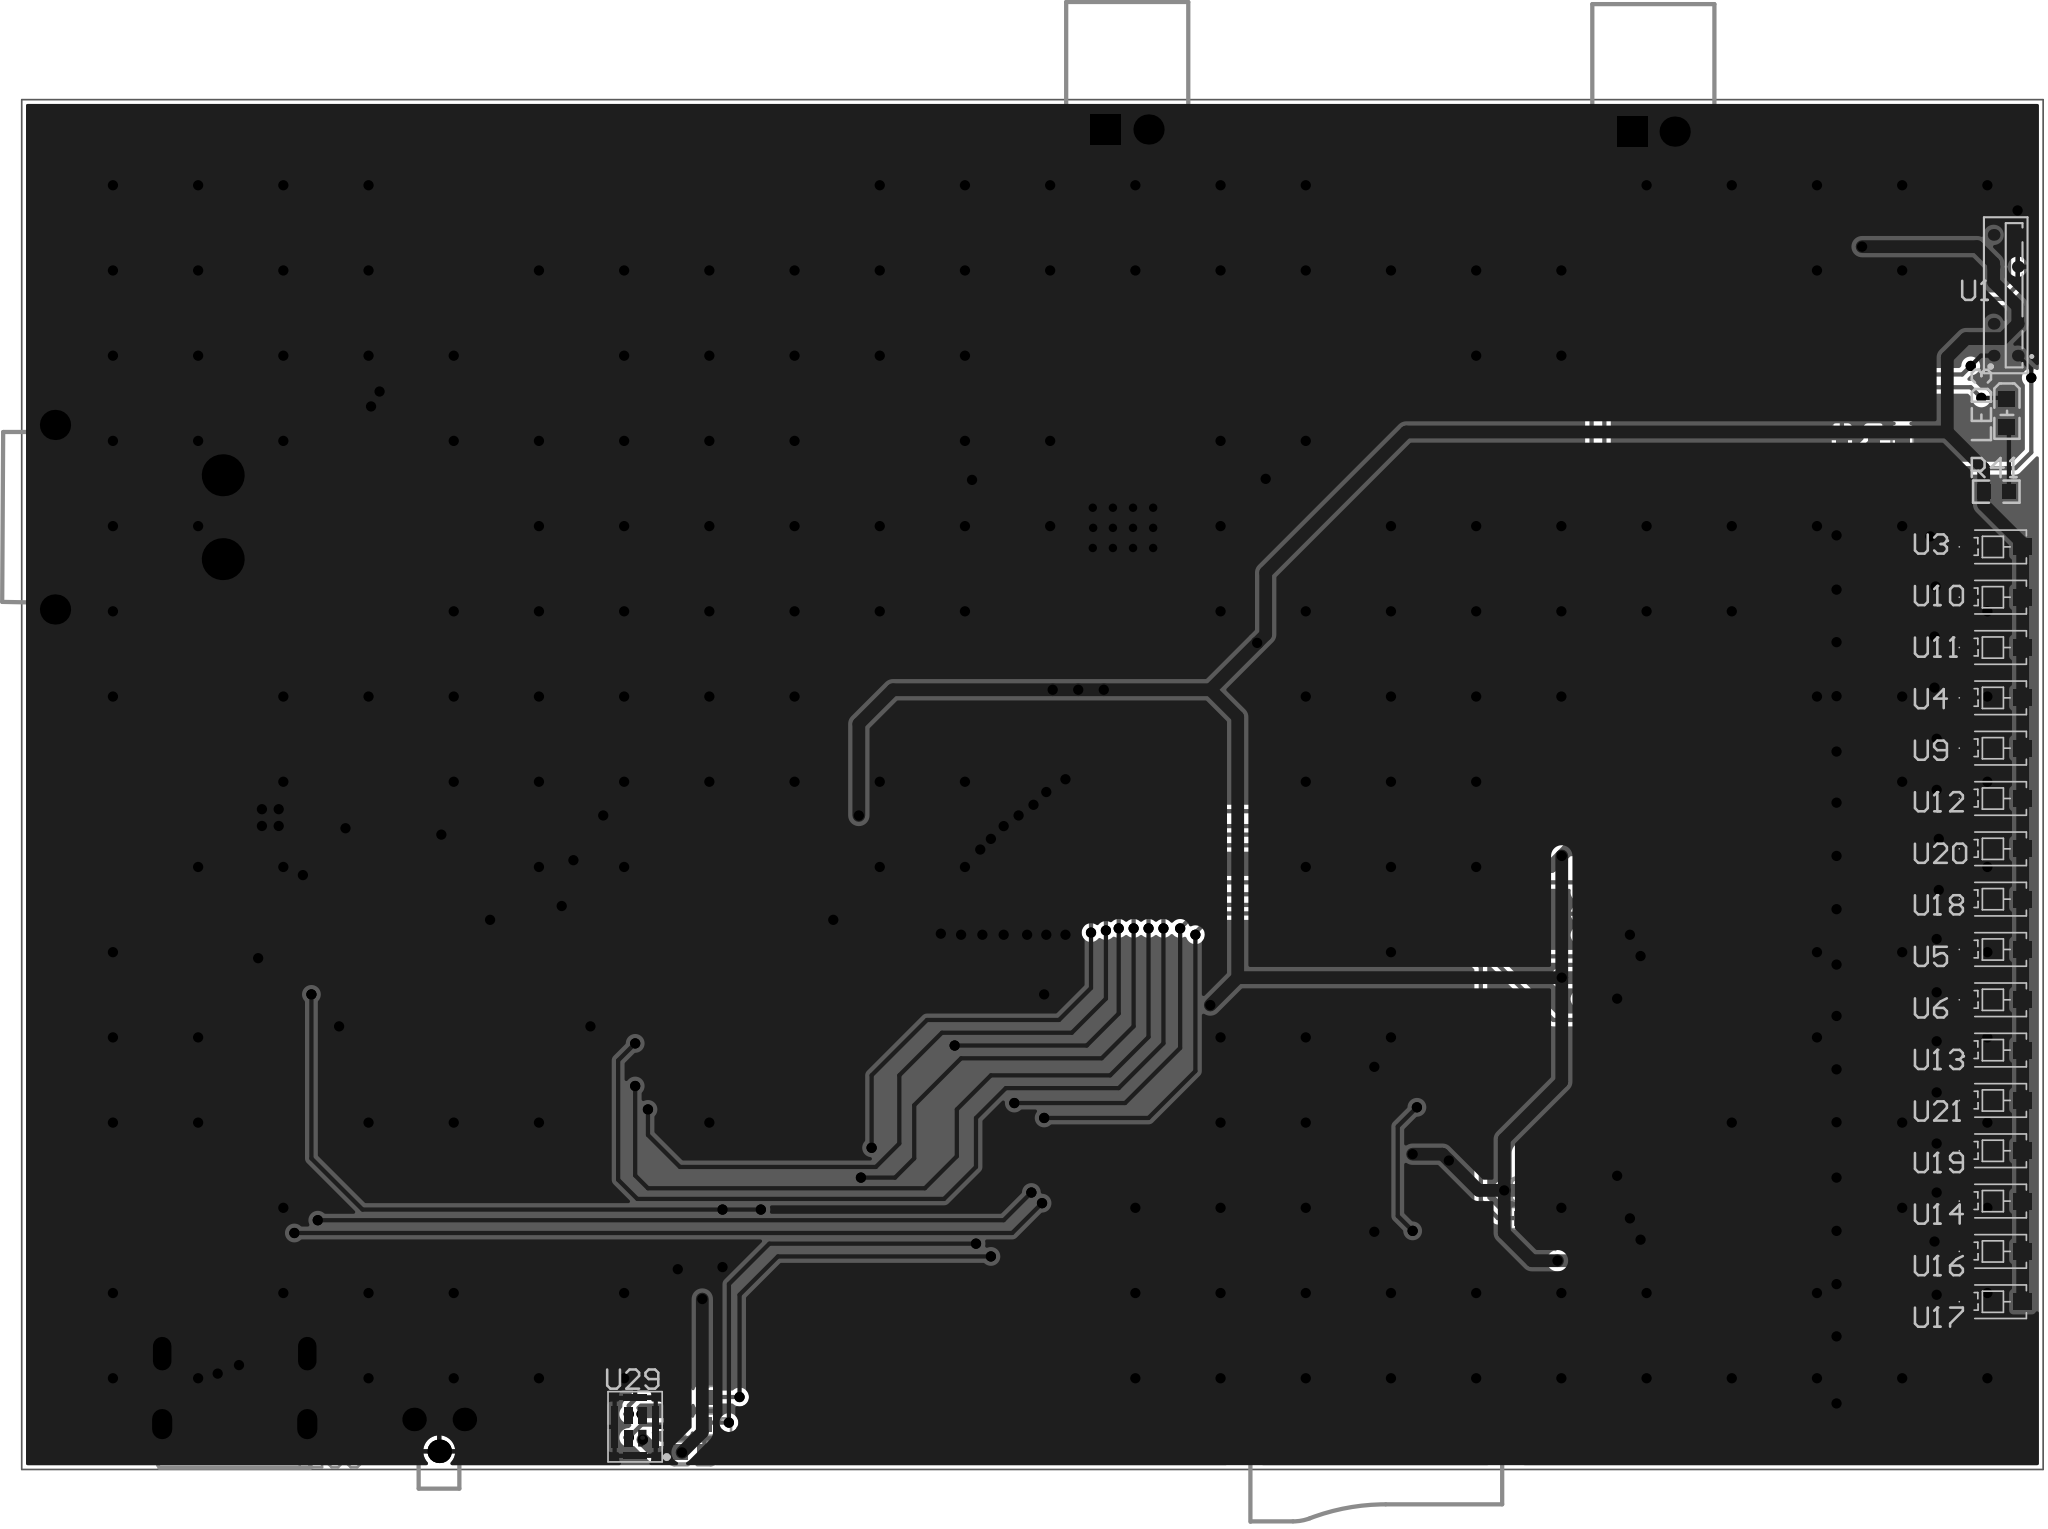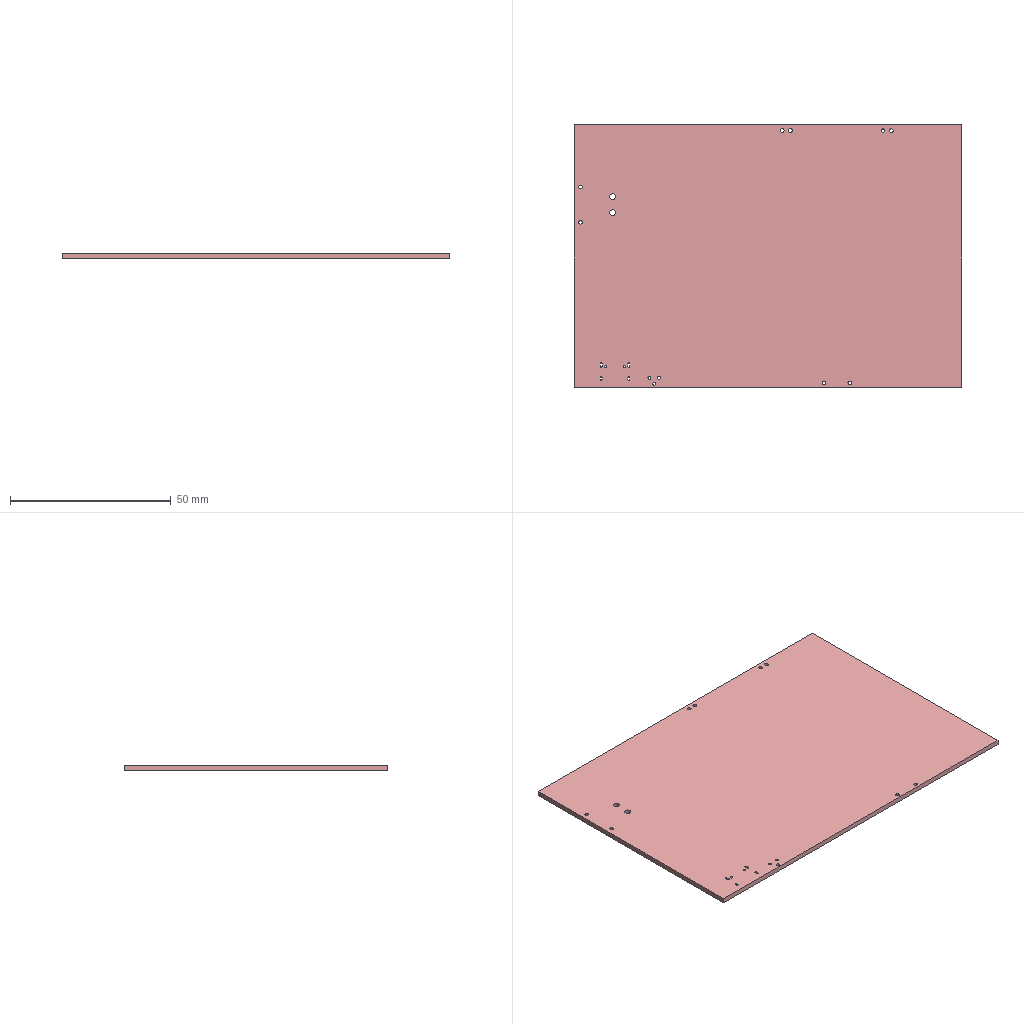Circuit board layout | Altium Designer | box 120.5 x 81.7 x 1.6 mm
Layer stack:
# Altium Designer layer stack of  (unit mm; dielectric type: 0 none, 1 core, 2 prepreg, 3 surface material)
index,name,kind,layer,copper_thickness_mm,dielectric_type,dielectric_thickness_mm,dielectric_material,dielectric_constant
0,Top Paste Mask Layer,other,,,,,,
1,Top Silkscreen Layer,other,,,,,,
2,Top Solder Mask Layer,dielectric,,,3,0.01,,3.3
3,Top Layer,copper,Top Layer,0.035,,,,
4,Dielectric1,dielectric,,,3,1.51,FR4,4.5
5,Bottom Layer,copper,Bottom Layer,0.035,,,,
6,Bottom Solder Mask Layer,dielectric,,,3,0.01,,3.3
7,Bottom Silkscreen Layer,other,,,,,,
8,Bottom Paste Mask Layer,other,,,,,,
# drill layer pairs: low layer,high layer
drill_pair,Top Layer,Bottom Layer
Part placement:
Designator,Comment,Layer,Footprint,Center-X(mm),Center-Y(mm),Rotation
Q1,2N7002,BottomLayer,SOT-23-3_L2.9-W1.3-P1.90-LS2.4-BR,193.548,136.779,180
Q2,2N7002,BottomLayer,SOT-23-3_L2.9-W1.3-P1.90-LS2.4-BR,193.548,127.229,180
Q3,2N7002,BottomLayer,SOT-23-3_L2.9-W1.3-P1.90-LS2.4-BR,193.548,111.311,180
Q4,2N7002,BottomLayer,SOT-23-3_L2.9-W1.3-P1.90-LS2.4-BR,193.548,108.128,180
Q5,2N7002,BottomLayer,SOT-23-3_L2.9-W1.3-P1.90-LS2.4-BR,193.548,124.045,180
Q6,2N7002,BottomLayer,SOT-23-3_L2.9-W1.3-P1.90-LS2.4-BR,193.548,133.595,180
Q7,2N7002,BottomLayer,SOT-23-3_L2.9-W1.3-P1.90-LS2.4-BR,193.548,130.412,180
Q8,2N7002,BottomLayer,SOT-23-3_L2.9-W1.3-P1.90-LS2.4-BR,193.548,120.862,180
Q9,2N7002,BottomLayer,SOT-23-3_L2.9-W1.3-P1.90-LS2.4-BR,193.548,104.944,180
Q10,2N7002,BottomLayer,SOT-23-3_L2.9-W1.3-P1.90-LS2.4-BR,193.548,95.394,180
Q11,2N7002,BottomLayer,SOT-23-3_L2.9-W1.3-P1.90-LS2.4-BR,193.548,92.21,180
Q12,2N7002,BottomLayer,SOT-23-3_L2.9-W1.3-P1.90-LS2.4-BR,193.548,89.027,180
Q13,2N7002,BottomLayer,SOT-23-3_L2.9-W1.3-P1.90-LS2.4-BR,193.548,114.495,180
Q14,2N7002,BottomLayer,SOT-23-3_L2.9-W1.3-P1.90-LS2.4-BR,193.548,98.577,180
Q15,2N7002,BottomLayer,SOT-23-3_L2.9-W1.3-P1.90-LS2.4-BR,193.548,117.678,180
Q16,2N7002,BottomLayer,SOT-23-3_L2.9-W1.3-P1.90-LS2.4-BR,193.548,101.761,180
U1,S13131-1536,TopLayer,BGA-8_L9.1-W2.4_S13131-1536,201.096,152.042,90
U3,TEMT6000X01,TopLayer,SENSORS-SMD_TEMT6000X01,200.327,137.042,0
U4,TEMT6000X01,TopLayer,SENSORS-SMD_TEMT6000X01,200.327,128.042,0
U5,TEMT6000X01,TopLayer,SENSORS-SMD_TEMT6000X01,200.327,113.042,0
U6,TEMT6000X01,TopLayer,SENSORS-SMD_TEMT6000X01,200.327,110.042,0
U7,74HC595,BottomLayer,SOP-16_L9.9-W3.9-P1.27-LS6.0-BL,179.197,114.537,270
U8,74HC595,BottomLayer,SOP-16_L9.9-W3.9-P1.27-LS6.0-BL,179.07,97.646,270
U9,TEMT6000X01,TopLayer,SENSORS-SMD_TEMT6000X01,200.327,125.042,0
U10,TEMT6000X01,TopLayer,SENSORS-SMD_TEMT6000X01,200.327,134.042,0
U11,TEMT6000X01,TopLayer,SENSORS-SMD_TEMT6000X01,200.327,131.042,0
U12,TEMT6000X01,TopLayer,SENSORS-SMD_TEMT6000X01,200.327,122.042,0
U13,TEMT6000X01,TopLayer,SENSORS-SMD_TEMT6000X01,200.327,107.042,0
U14,TEMT6000X01,TopLayer,SENSORS-SMD_TEMT6000X01,200.327,98.042,0
U16,TEMT6000X01,TopLayer,SENSORS-SMD_TEMT6000X01,200.327,95.042,0
U17,TEMT6000X01,TopLayer,SENSORS-SMD_TEMT6000X01,200.327,92.042,0
U18,TEMT6000X01,TopLayer,SENSORS-SMD_TEMT6000X01,200.327,116.042,0
U19,TEMT6000X01,TopLayer,SENSORS-SMD_TEMT6000X01,200.327,101.042,0
U20,TEMT6000X01,TopLayer,SENSORS-SMD_TEMT6000X01,200.327,119.042,0
U21,TEMT6000X01,TopLayer,SENSORS-SMD_TEMT6000X01,200.327,104.042,0
U22,LMV321IDBVR,BottomLayer,SOT-23-5_L3.0-W1.7-P0.95-LS2.8-BR,193.802,150.876,0
C1,100nF,BottomLayer,C0603,172.466,117.983,180
C2,100nF,BottomLayer,C0603,172.974,98.679,0
C3,100nF,BottomLayer,C0603,190.562,151.048,270
C4,22pF,BottomLayer,C0603,85.344,98.298,90
C5,22pF,BottomLayer,C0603,88.903,95.123,0
C6,10uF,BottomLayer,C0603,91.339,124.269,180
C7,22uF,BottomLayer,C0603,91.339,126.047,180
C8,22uF,BottomLayer,C0603,115.062,120.142,0
C9,22uF,BottomLayer,C0603,91.189,118.491,0
C10,10uF,BottomLayer,C0603,91.313,129.54,0
C11,100nF,BottomLayer,C0603,161.544,98.552,90
C12,100nF,BottomLayer,C0603,114.3,96.52,180
C13,1uF,BottomLayer,C0603,122.682,95.377,0
C14,1uF,BottomLayer,C0603,138.43,116.332,90
C15,10uF,BottomLayer,C0603,100.584,140.843,180
C16,100nF,BottomLayer,C0603,115.059,121.92,180
C17,2.2uF,BottomLayer,CAP-SMD_BD5.0-L5.3-W5.3-LS6.0-FD,115.276,139.344,90
C18,100nF,BottomLayer,C0603,101.6,136.017,270
C19,1uF,BottomLayer,C0603,103.973,151.282,180
C20,22uF,BottomLayer,C0603,112.649,146.05,180
C21,33pF,BottomLayer,C0603,112.609,149.377,0
C22,47nF,BottomLayer,C0603,100.711,142.494,180
C23,22uF,BottomLayer,CAP-SMD_BD5.0-L5.3-W5.3-LS6.3-FD-1,115.189,158.242,270
C24,22uF,BottomLayer,CAP-SMD_BD5.0-L5.3-W5.3-LS6.3-FD-1,121.539,158.369,270
C25,22uF,BottomLayer,CAP-SMD_BD5.0-L5.3-W5.3-LS6.3-FD-1,127.762,158.369,270
C26,100nF,BottomLayer,C0603,154.178,130.429,270
C27,1uF,BottomLayer,C0603,150.622,130.429,270
C28,1uF,BottomLayer,C0603,142.621,130.429,90
C29,220uF,BottomLayer,CAP-SMD_BD6.3-L6.6-W6.6-LS7.3-FD-H7.7,108.204,157.988,270
C30,680nF,BottomLayer,C0603,178.181,155.829,180
C31,10uF,BottomLayer,C0603,155.321,140.462,90
C32,100nF,BottomLayer,C0603,141.478,140.335,90
C37,680nF,BottomLayer,C0603,182.499,155.702,180
C38,680nF,BottomLayer,C0603,146.431,155.448,180
C39,680nF,BottomLayer,C0603,150.495,155.448,180
C40,100nF,BottomLayer,C0603,122.806,83.058,0
CARD2,TF-15x15,BottomLayer,TF-SMD_TF-15-15,163.703,89.027,270
CN1,XT30PW-M30.G.Y,BottomLayer,CONN-TH_XT30PW-M,89.789,138.811,90
CN2,S2B-XH-A-1(LF)(SN),BottomLayer,CONN-TH_S2B-XH-A-1-LF-SN,180.086,161.798,180
CN3,S2B-XH-A-1(LF)(SN),BottomLayer,CONN-TH_S2B-XH-A-1-LF-SN,148.717,161.925,180
D1,1N4148W,BottomLayer,SOD-123_L2.7-W1.6-LS3.7-FD,113.411,94.361,0
D2,1N4148W,BottomLayer,SOD-123_L2.7-W1.6-LS3.7-FD,113.238,91.313,180
L1,2.2uH,BottomLayer,IND-SMD_L4.6-W4.1_MHCI04015,105.497,134.772,270
L2,10uH,BottomLayer,IND-SMD_L7.3-W6.8,171.415,158.242,90
L3,10uH,BottomLayer,IND-SMD_L7.3-W6.8,188.94,158.242,90
L4,10uH,BottomLayer,IND-SMD_L7.3-W6.8,139.918,158.496,90
L5,10uH,BottomLayer,IND-SMD_L7.3-W6.8,157.445,158.496,90
LED1,NCD0603Y2,BottomLayer,LED0603-RD,104.114,124.968,0
LED2,NCD0603Y2,BottomLayer,LED0603-RD,97.79,115.57,270
LED3,GL0603UR01,TopLayer,LED0603-FD,201.168,145.034,90
Q17,UMH3N,BottomLayer,SC-70-6_L2.2-W1.3-P0.65-LS2.1-BR,98.298,110.617,270
Q18,2N7002,BottomLayer,SOT-23-3_L2.9-W1.3-P1.90-LS2.4-BR,109.728,97.028,180
Q19,2N7002,BottomLayer,SOT-23-3_L2.9-W1.3-P1.90-LS2.4-BR,192.278,144.526,270
R1,10kΩ,BottomLayer,R0603,193.421,85.979,0
R2,49.9Ω,BottomLayer,R0603,193.929,148.336,180
R3,10kΩ,BottomLayer,R0603,151.892,110.507,270
R4,5.1kΩ,BottomLayer,R0603,96.774,92.583,270
R5,27Ω,BottomLayer,R0603,95.25,97.79,270
R6,27Ω,BottomLayer,R0603,96.774,97.79,270
R7,5.1kΩ,BottomLayer,R0603,93.726,92.583,270
R8,49.9Ω,BottomLayer,R0603,122.682,105.156,180
R9,49.9Ω,BottomLayer,R0603,172.974,97.028,0
R10,49.9Ω,BottomLayer,R0603,122.682,107.442,0
R11,49.9Ω,BottomLayer,R0603,122.682,103.632,0
R12,49.9Ω,BottomLayer,R0603,193.912,141.732,180
R13,10kΩ,BottomLayer,R0603,122.682,97.536,0
R14,1kΩ,BottomLayer,R0603,104.14,121.548,180
R15,82kΩ,BottomLayer,R0603,104.14,116.967,180
R16,47kΩ,BottomLayer,R0603,91.186,120.269,180
R17,100Ω,BottomLayer,R0603,104.14,123.19,180
R18,HNTC0805-104F3950FB,BottomLayer,R0805,104.14,118.999,180
R19,2Ω,BottomLayer,R0603,91.313,127.762,180
R20,500mΩ,BottomLayer,R1206,93.472,115.951,0
R21,100Ω,BottomLayer,R0603,99.568,115.57,90
R22,4.7kΩ,BottomLayer,R0603,163.449,98.552,270
R23,4.7kΩ,BottomLayer,R0603,165.735,98.552,270
R24,4.7kΩ,BottomLayer,R0603,167.894,98.552,270
R25,1MΩ,BottomLayer,R0603,117.475,94.361,0
R26,10kΩ,BottomLayer,R0603,117.429,91.313,180
R27,100kΩ,BottomLayer,R0603,109.601,94.361,0
R28,499kΩ,BottomLayer,R0603,136.516,116.214,90
R29,100kΩ,BottomLayer,R0603,135.001,116.205,270
R30,249kΩ,BottomLayer,R0603,109.307,137.312,270
R31,20kΩ,BottomLayer,R0603,109.942,151.282,180
R32,180kΩ,BottomLayer,R0603,106.934,151.257,180
R33,100kΩ,BottomLayer,R0603,112.609,144.297,180
R34,10kΩ,BottomLayer,R0603,112.609,147.726,0
R35,4.7kΩ,BottomLayer,R0603,152.4,130.429,90
R36,10kΩ,BottomLayer,R0603,144.272,130.429,90
R37,2.2kΩ,BottomLayer,R0603,147.32,130.429,90
R38,2.2kΩ,BottomLayer,R0603,145.796,130.429,90
R39,33Ω,BottomLayer,R0603,122.826,86.36,180
R40,33Ω,BottomLayer,R0603,122.8,84.718,180
R41,56Ω,TopLayer,R0603,200.533,140.335,0
R42,10kΩ,BottomLayer,R0603,194.945,144.399,90
SW1,TS-1088-AR02016,BottomLayer,SW-SMD_L3.9-W3.0-P4.45,122.301,100.457,0
SW2,TS-1088-AR02016,BottomLayer,SW-SMD_L3.9-W3.0-P4.45,157.988,111.76,0
U2,CH340G,BottomLayer,SOIC-16_L9.9-W3.9-P1.27-LS6.0-BL,97.282,103.632,180
U15,ESP32-S3-WROOM-1-N8R8,BottomLayer,WIRELM-SMD_ESP32-S3-WROOM-1,138.176,103.632,0
U23,IP2312U_VSET,BottomLayer,SOP-8_L4.9-W3.9-P1.27-LS6.0-BL-EP,97.626,120.904,270
U24,1uH,BottomLayer,IND-SMD_L2.5-W2.0-VLS252012CX-150M,91.313,122.174,180
U26,ME6211A33M3G-N,BottomLayer,SOT-23-3_L2.9-W1.6-P1.90-LS2.8-BR,135.382,120.142,180
U27,TAS5805MPWPR,BottomLayer,HTSSOP-28_L9.7-W4.4-P0.65-LS6.4-BL-EP,148.463,138.176,180
U28,TPS61088RHLR,BottomLayer,VQFN-20_L4.6-W3.6-P0.50-BL,105.624,142.646,180
U29,MSM261DHP006,TopLayer,QFN-8_L4.0-W3.0_WMM7040DTHN0-8-TR,119.38,84.582,0
USB1,TYPE-C 16PIN 2MD(073),BottomLayer,USB-C-SMD_TYPE-C-6PIN-2MD-073,95.504,87.122,180
X1,12MHz,BottomLayer,CRYSTAL-SMD_4P-L3.2-W2.5-BL,88.544,98.171,180
C33,220nF,BottomLayer,C0603,143.637,149.606,180
C34,220nF,BottomLayer,C0603,148.844,149.352,180
C35,220nF,BottomLayer,C0603,153.543,148.971,0
C36,220nF,BottomLayer,C0603,157.353,149.098,0
SW3,TS-1009B-05026,BottomLayer,SW-TH_3P-L4.5-W3.8-P3.10-LS1.9_TS-1009B-05026,107.696,84.074,180
U30,TPS22965DSGR,BottomLayer,UDFN-8_L2.0-W2.0-P0.50-TL-EP,119.547,120.681,0
C41,1nF,BottomLayer,C0603,123.698,120.904,0
Pad and via stacks:
# Altium Designer via and pad stacks of  (unit mm). Each distinct definition once, with the count of objects using it.
# via: kind,start_layer,end_layer,hole_mm,diameter_mm,mode(0 simple;1 top-mid-bottom;2 full stack),diameter_per_layer,count,example_net
# pad: kind,layer,hole_mm,hole_type(0 round;1 square;2 slot),plating,top_size,top_shape(1 round;2 rect;3 octagon;9 rounded rect),mid_size,bottom_size,mode,footprint,size_per_layer,count,example
pad,Bottom Layer,0,0,plated,1.25x0.7,2,1.25x0.7,1.25x0.7,0,SOT-23-3_L2.9-W1.3-P1.90-LS2.4-BR,,54,Q1.1
pad,Bottom Layer,0,0,plated,0.574x2.038,1,0.574x2.038,0.574x2.038,0,SOP-16_L9.9-W3.9-P1.27-LS6.0-BL,,32,U7.1
pad,Bottom Layer,0,0,plated,1.1x0.6,2,1.1x0.6,1.1x0.6,0,SOT-23-5_L3.0-W1.7-P0.95-LS2.8-BR,,5,U22.5
pad,Bottom Layer,0,0,plated,0.8x0.9,2,0.8x0.9,0.8x0.9,0,C0603,,72,C1.2
pad,Bottom Layer,0,0,plated,2.8x1.1,2,2.8x1.1,2.8x1.1,0,CAP-SMD_BD5.0-L5.3-W5.3-LS6.0-FD,,2,C17.2
pad,Bottom Layer,0,0,plated,2.7x0.91,2,2.7x0.91,2.7x0.91,0,CAP-SMD_BD5.0-L5.3-W5.3-LS6.3-FD-1,,6,C23.2
pad,Bottom Layer,0,0,plated,3.5x1.2,2,3.5x1.2,3.5x1.2,0,CAP-SMD_BD6.3-L6.6-W6.6-LS7.3-FD-H7.7,,2,C29.1
pad,Bottom Layer,0,0,plated,1.6x0.701,2,1.6x0.701,1.6x0.701,0,TF-SMD_TF-15-15,,9,CARD2.1
pad,Bottom Layer,0,0,plated,1.6x1.8,2,1.6x1.8,1.6x1.8,0,TF-SMD_TF-15-15,,1,CARD2.10
pad,Bottom Layer,0,0,plated,2.4x1.6,2,2.4x1.6,2.4x1.6,0,TF-SMD_TF-15-15,,2,CARD2.11
pad,Bottom Layer,0,0,plated,1.399x1.801,2,1.399x1.801,1.399x1.801,0,TF-SMD_TF-15-15,,1,CARD2.13
pad,Bottom Layer,0,0,plated,0.88x0.96,2,0.88x0.96,0.88x0.96,0,SOD-123_L2.7-W1.6-LS3.7-FD,,4,D1.1
pad,Bottom Layer,0,0,plated,2.5x1.5,2,2.5x1.5,2.5x1.5,0,IND-SMD_L4.6-W4.1_MHCI04015,,2,L1.1
pad,Bottom Layer,0,0,plated,2.35x3.5,2,2.35x3.5,2.35x3.5,0,IND-SMD_L7.3-W6.8,,8,L2.2
pad,Bottom Layer,0,0,plated,0.8x0.8,2,0.8x0.8,0.8x0.8,0,LED0603-RD,,4,LED1.2
pad,Bottom Layer,0,0,plated,0.42x0.6,2,0.42x0.6,0.42x0.6,0,SC-70-6_L2.2-W1.3-P0.65-LS2.1-BR,,6,Q17.6
pad,Bottom Layer,0,0,plated,0.8065x0.864,2,0.8065x0.864,0.8065x0.864,0,R0603,,78,R1.2
pad,Bottom Layer,0,0,plated,1.133x1.377,2,1.133x1.377,1.133x1.377,0,R0805,,2,R18.2
pad,Bottom Layer,0,0,plated,1.208x1.701,2,1.208x1.701,1.208x1.701,0,R1206,,2,R20.2
pad,Bottom Layer,0,0,plated,1.23x1.86,2,1.23x1.86,1.23x1.86,0,SW-SMD_L3.9-W3.0-P4.45,,4,SW1.1
pad,Bottom Layer,0,0,plated,0.602x1.971,1,0.602x1.971,0.602x1.971,0,SOIC-16_L9.9-W3.9-P1.27-LS6.0-BL,,16,U2.1
pad,Bottom Layer,0,0,plated,1.5x0.9,2,1.5x0.9,1.5x0.9,0,WIRELM-SMD_ESP32-S3-WROOM-1,,40,U15.1
pad,Bottom Layer,0,0,plated,0.9x0.9,2,0.9x0.9,0.9x0.9,0,WIRELM-SMD_ESP32-S3-WROOM-1,,9,U15.41
pad,Bottom Layer,0,0,plated,0.6x1.8,1,0.6x1.8,0.6x1.8,0,SOP-8_L4.9-W3.9-P1.27-LS6.0-BL-EP,,8,U23.1
pad,Bottom Layer,0,0,plated,2.29x2.29,2,2.29x2.29,2.29x2.29,0,SOP-8_L4.9-W3.9-P1.27-LS6.0-BL-EP,,1,U23.9
pad,Bottom Layer,0,0,plated,0.85x2,2,0.85x2,0.85x2,0,IND-SMD_L2.5-W2.0-VLS252012CX-150M,,2,U24.2
pad,Bottom Layer,0,0,plated,1.07x0.6,2,1.07x0.6,1.07x0.6,0,SOT-23-3_L2.9-W1.6-P1.90-LS2.8-BR,,3,U26.1
pad,Bottom Layer,0,0,plated,0.343x1.732,1,0.343x1.732,0.343x1.732,0,HTSSOP-28_L9.7-W4.4-P0.65-LS6.4-BL-EP,,28,U27.1
pad,Bottom Layer,0,0,plated,5.6x3.1,2,5.6x3.1,5.6x3.1,0,HTSSOP-28_L9.7-W4.4-P0.65-LS6.4-BL-EP,,1,U27.29
pad,Bottom Layer,0,0,plated,0.2438x0.7,2,0.2438x0.7,0.2438x0.7,0,VQFN-20_L4.6-W3.6-P0.50-BL,,16,U28.2
pad,Bottom Layer,0,0,plated,0.7x0.2438,2,0.7x0.2438,0.7x0.2438,0,VQFN-20_L4.6-W3.6-P0.50-BL,,4,U28.10
pad,Bottom Layer,0,0,plated,1.015x1.015,1,1.015x1.015,1.015x1.015,0,VQFN-20_L4.6-W3.6-P0.50-BL,,1,U28.21
pad,Bottom Layer,0,0,plated,0.55x1.1,2,0.55x1.1,0.55x1.1,0,USB-C-SMD_TYPE-C-6PIN-2MD-073,,4,USB1.1
pad,Bottom Layer,0,0,plated,0.3x1.1,2,0.3x1.1,0.3x1.1,0,USB-C-SMD_TYPE-C-6PIN-2MD-073,,8,USB1.3
pad,Bottom Layer,0,0,plated,1.4x1.2,2,1.4x1.2,1.4x1.2,0,CRYSTAL-SMD_4P-L3.2-W2.5-BL,,4,X1.1
pad,Bottom Layer,0,0,plated,0.505x0.28,2,0.505x0.28,0.505x0.28,0,UDFN-8_L2.0-W2.0-P0.50-TL-EP,,8,U30.1
pad,Bottom Layer,0,0,plated,0.9x1.7,2,0.9x1.7,0.9x1.7,0,UDFN-8_L2.0-W2.0-P0.50-TL-EP,,1,U30.9
pad,Top Layer,0,0,plated,0.7x0.7,1,0.7x0.7,0.7x0.7,0,BGA-8_L9.1-W2.4_S13131-1536,,8,U1.8
pad,Top Layer,0,0,plated,1.1x1.001,2,1.1x1.001,1.1x1.001,0,SENSORS-SMD_TEMT6000X01,,16,U3.3
pad,Top Layer,0,0,plated,1.1x0.8001,2,1.1x0.8001,1.1x0.8001,0,SENSORS-SMD_TEMT6000X01,,32,U3.1
pad,Top Layer,0,0,plated,1x0.8999,2,1x0.8999,1x0.8999,0,LED0603-FD,,2,LED3.1
pad,Top Layer,0,0,plated,0.8065x0.864,2,0.8065x0.864,0.8065x0.864,0,R0603,,2,R41.2
pad,Top Layer,0,0,plated,0.5x1,2,0.5x1,0.5x1,0,QFN-8_L4.0-W3.0_WMM7040DTHN0-8-TR,,3,U29.4
pad,Top Layer,0,0,plated,0.2389x0.2389,1,0.2389x0.2389,0.2389x0.2389,0,QFN-8_L4.0-W3.0_WMM7040DTHN0-8-TR,,1,U29.1
pad,Top Layer,0,0,plated,0.4x2.5,2,0.4x2.5,0.4x2.5,0,QFN-8_L4.0-W3.0_WMM7040DTHN0-8-TR,,2,U29.8
pad,Top Layer,0,0,plated,0.4x1.4,2,0.4x1.4,0.4x1.4,0,QFN-8_L4.0-W3.0_WMM7040DTHN0-8-TR,,2,U29.7
pad,Multi-Layer,1.8,0,plated,2.5x2.5,1,2.5x2.5,2.5x2.5,0,CONN-TH_XT30PW-M,,2,CN1.1
pad,Multi-Layer,1.1,0,plated,1.8x1.8,1,1.8x1.8,1.8x1.8,0,CONN-TH_XT30PW-M,,2,CN1.3
pad,Multi-Layer,1.2,0,plated,1.8x1.8,2,1.8x1.8,1.8x1.8,0,CONN-TH_S2B-XH-A-1-LF-SN,,2,CN2.1
pad,Multi-Layer,1.2,0,plated,1.8x1.8,1,1.8x1.8,1.8x1.8,0,CONN-TH_S2B-XH-A-1-LF-SN,,2,CN2.2
pad,Multi-Layer,0.6,2,plated,1.1x2,1,1.1x2,1.1x2,0,USB-C-SMD_TYPE-C-6PIN-2MD-073,,2,USB1.13
pad,Multi-Layer,0.6,2,plated,1.2x1.8,1,1.2x1.8,1.2x1.8,0,USB-C-SMD_TYPE-C-6PIN-2MD-073,,2,USB1.13
pad,Multi-Layer,0.9,0,plated,1.4x1.4,1,1.4x1.4,1.4x1.4,0,SW-TH_3P-L4.5-W3.8-P3.10-LS1.9_TS-1009B-05026,,3,SW3.1
via,Top Layer,Bottom Layer,0.3048,0.6096,0,,4,AGND
via,Top Layer,Bottom Layer,0.2997,0.5,0,,12,AGND
via,Top Layer,Bottom Layer,0.3048,0.61,0,,317,RESET
Copper pours:
name,layer,net,type(0 solid;1 hatched;2 none)
Bottom Layer-AGND,Bottom Layer,AGND,0
Top Layer-AGND,Top Layer,AGND,0
Design rules, without the lines most boards share:
# Altium Designer design rules of  (exported by Altium Designer, unit mm)
# columns: name | kind | enabled | priority | scope1 | scope2 | descriptor | typed fields (field=value)
copperThickness2oz | 0 | enabled | 1 | (InNet('OUT_A-') OR InNet('OUT_A+') OR InNet('OUT_B-') OR InNet('OUT_B+')) | All | Clearance Constraint (Gap=5.984mil) ((InNet('OUT_A-') OR InNet('OUT_A+') OR InNet('OUT_B-') OR InNet('OUT_B+'))),(All) | gap=0.152
copperThickness2oz_1 | 63 | enabled | 1 | All | All | Board Clearance Constraint (Gap=0mil) (All) |
copperThickness1oz_2 | 2 | disabled | 1 | All | All | Width Constraint (Min=5mil) (Max=100mil) (Preferred=10mil) (Disabled)(All) |
power_trackWidth1 | 2 | disabled | 2 | All | All | Width Constraint (Min=23.6mil) (Max=78.7mil) (Preferred=39.4mil) (Disabled)(All) |
trackWidth2 | 2 | enabled | 3 | (InNet('+12V') OR InNet('OUT_A-') OR InNet('OUT_A+') OR InNet('OUT_B-') OR InNet('OUT_B+') OR InNet('VBUS') OR InNet('VSYS_MAIN')) | All | Width Constraint (Min=15.7mil) (Max=39.4mil) (Preferred=19.7mil) ((InNet('+12V') OR InNet('OUT_A-') OR InNet('OUT_A+') OR InNet('OUT_B-') OR InNet('OUT_B+') OR InNet('VBUS') OR InNet('VSYS_MAIN'))) |
trackWidth3_BAT | 2 | enabled | 4 | (InNet('VBAT')) | All | Width Constraint (Min=15.7mil) (Max=100mil) (Preferred=59.1mil) ((InNet('VBAT'))) |
copperThickness2oz_2 | 2 | enabled | 5 | All | All | Width Constraint (Min=8mil) (Max=100mil) (Preferred=10mil) (All) |
copperRegion | 20 | enabled | 1 | (InNet('PD_GATE_15') OR InNet('IO0')) | All | Polygon Connect Rule(Relief Connect )(Conductor Width=10mil) (Relief Angle=90 Angle) (Entries=4) (Air Gap Width=10mil) ((InNet('PD_GATE_15') OR InNet('IO0'))),(All) | connect_style(0=relief,1=direct,2=none)=0 relief_conductor_width=0.254 relief_entries=4